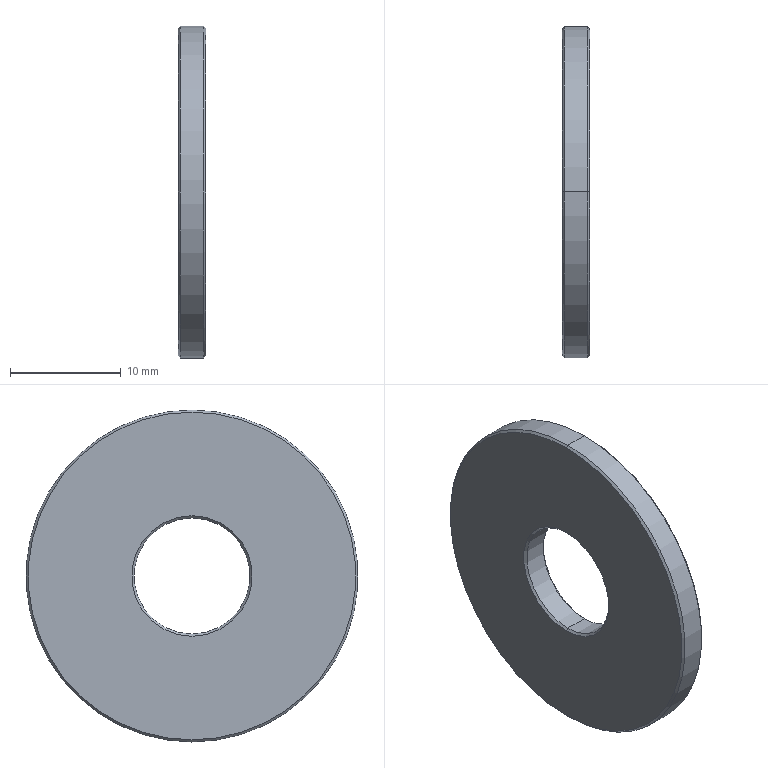Part | STEP file | WSX-SUS-M10X30-2.5-5 | 1 solid | 14 faces | box 2.5 x 30 x 30 mm | volume 1546 mm3 | cone 8 | cylinder 4 | plane 2 | commonest cylinder face diameters 10.5 x2 30 x2
STEP:
#1=CARTESIAN_POINT('',(0.,0.,0.));
#2=DIRECTION('',(0.,0.,1.));
#3=DIRECTION('',(1.,0.,0.));
#4=AXIS2_PLACEMENT_3D('',#1,#2,#3);
#5=CARTESIAN_POINT('',(2.5,0.,-14.8));
#6=VERTEX_POINT('',#5);
#7=CARTESIAN_POINT('',(2.5,0.,14.8));
#8=VERTEX_POINT('',#7);
#9=CARTESIAN_POINT('',(2.5,0.,0.));
#10=DIRECTION('',(1.,0.,0.));
#11=DIRECTION('',(0.,0.,1.));
#12=AXIS2_PLACEMENT_3D('',#9,#10,#11);
#13=CIRCLE('',#12,14.8);
#14=CARTESIAN_POINT('',(2.3,0.,0.));
#15=DIRECTION('',(-1.,0.,0.));
#16=DIRECTION('',(0.,0.,1.));
#17=AXIS2_PLACEMENT_3D('',#14,#15,#16);
#18=CONICAL_SURFACE('',#17,15.,0.7854);
#19=CARTESIAN_POINT('',(6.283,-0.2));
#20=DIRECTION('',(-1.,0.));
#21=VECTOR('',#20,1.);
#22=LINE('',#19,#21);
#23=(GEOMETRIC_REPRESENTATION_CONTEXT(2)PARAMETRIC_REPRESENTATION_CONTEXT()REPRESENTATION_CONTEXT('',''));
#24=DEFINITIONAL_REPRESENTATION('',(#22),#23);
#25=PCURVE('',#18,#24);
#26=CARTESIAN_POINT('',(2.5,5.,0.));
#27=DIRECTION('',(-1.,0.,0.));
#28=DIRECTION('',(0.,0.,1.));
#29=AXIS2_PLACEMENT_3D('',#26,#27,#28);
#30=PLANE('',#29);
#31=CARTESIAN_POINT('',(14.8,-5.));
#32=CARTESIAN_POINT('',(14.8,-30.634));
#33=CARTESIAN_POINT('',(-7.4,-17.817));
#34=CARTESIAN_POINT('',(-29.6,-5.));
#35=CARTESIAN_POINT('',(-7.4,7.817));
#36=CARTESIAN_POINT('',(14.8,20.634));
#37=CARTESIAN_POINT('',(14.8,-5.));
#38=(BOUNDED_CURVE()B_SPLINE_CURVE(2,(#31,#32,#33,#34,#35,#36,#37),.UNSPECIFIED.,.T.,.F.)B_SPLINE_CURVE_WITH_KNOTS((1,2,2,2,2,1),(-2.094,0.,2.094,4.189,6.283,8.378),.UNSPECIFIED.)CURVE()GEOMETRIC_REPRESENTATION_ITEM()RATIONAL_B_SPLINE_CURVE((1.,0.5,1.,0.5,1.,0.5,1.))REPRESENTATION_ITEM(''));
#39=(GEOMETRIC_REPRESENTATION_CONTEXT(2)PARAMETRIC_REPRESENTATION_CONTEXT()REPRESENTATION_CONTEXT('',''));
#40=DEFINITIONAL_REPRESENTATION('',(#38),#39);
#41=PCURVE('',#30,#40);
#42=SURFACE_CURVE('',#13,(#25,#41),.PCURVE_S1.);
#43=EDGE_CURVE('',#6,#8,#42,.T.);
#44=ORIENTED_EDGE('',*,*,#43,.F.);
#45=CARTESIAN_POINT('',(2.3,0.,-15.));
#46=VERTEX_POINT('',#45);
#47=CARTESIAN_POINT('',(2.3,0.,-15.));
#48=DIRECTION('',(-0.7071,0.,-0.7071));
#49=VECTOR('',#48,1.);
#50=LINE('',#47,#49);
#51=CARTESIAN_POINT('',(3.142,0.));
#52=DIRECTION('',(0.,1.));
#53=VECTOR('',#52,1.);
#54=LINE('',#51,#53);
#55=(GEOMETRIC_REPRESENTATION_CONTEXT(2)PARAMETRIC_REPRESENTATION_CONTEXT()REPRESENTATION_CONTEXT('',''));
#56=DEFINITIONAL_REPRESENTATION('',(#54),#55);
#57=PCURVE('',#18,#56);
#58=CARTESIAN_POINT('',(2.3,0.,0.));
#59=DIRECTION('',(-1.,0.,0.));
#60=DIRECTION('',(0.,0.,1.));
#61=AXIS2_PLACEMENT_3D('',#58,#59,#60);
#62=CONICAL_SURFACE('',#61,15.,0.7854);
#63=CARTESIAN_POINT('',(3.142,0.));
#64=DIRECTION('',(0.,1.));
#65=VECTOR('',#64,1.);
#66=LINE('',#63,#65);
#67=(GEOMETRIC_REPRESENTATION_CONTEXT(2)PARAMETRIC_REPRESENTATION_CONTEXT()REPRESENTATION_CONTEXT('',''));
#68=DEFINITIONAL_REPRESENTATION('',(#66),#67);
#69=PCURVE('',#62,#68);
#70=SURFACE_CURVE('',#50,(#57,#69),.PCURVE_S1.);
#71=EDGE_CURVE('',#6,#46,#70,.T.);
#72=ORIENTED_EDGE('',*,*,#71,.T.);
#73=CARTESIAN_POINT('',(2.3,0.,15.));
#74=VERTEX_POINT('',#73);
#75=CARTESIAN_POINT('',(2.3,0.,0.));
#76=DIRECTION('',(-1.,0.,0.));
#77=DIRECTION('',(0.,0.,1.));
#78=AXIS2_PLACEMENT_3D('',#75,#76,#77);
#79=CIRCLE('',#78,15.);
#80=CARTESIAN_POINT('',(0.,0.));
#81=DIRECTION('',(1.,0.));
#82=VECTOR('',#81,1.);
#83=LINE('',#80,#82);
#84=(GEOMETRIC_REPRESENTATION_CONTEXT(2)PARAMETRIC_REPRESENTATION_CONTEXT()REPRESENTATION_CONTEXT('',''));
#85=DEFINITIONAL_REPRESENTATION('',(#83),#84);
#86=PCURVE('',#18,#85);
#87=CARTESIAN_POINT('',(0.,0.,0.));
#88=DIRECTION('',(-1.,0.,0.));
#89=DIRECTION('',(0.,0.,1.));
#90=AXIS2_PLACEMENT_3D('',#87,#88,#89);
#91=CYLINDRICAL_SURFACE('',#90,15.);
#92=CARTESIAN_POINT('',(0.,-2.3));
#93=DIRECTION('',(1.,0.));
#94=VECTOR('',#93,1.);
#95=LINE('',#92,#94);
#96=(GEOMETRIC_REPRESENTATION_CONTEXT(2)PARAMETRIC_REPRESENTATION_CONTEXT()REPRESENTATION_CONTEXT('',''));
#97=DEFINITIONAL_REPRESENTATION('',(#95),#96);
#98=PCURVE('',#91,#97);
#99=SURFACE_CURVE('',#79,(#86,#98),.PCURVE_S1.);
#100=EDGE_CURVE('',#74,#46,#99,.T.);
#101=ORIENTED_EDGE('',*,*,#100,.F.);
#102=CARTESIAN_POINT('',(2.3,0.,15.));
#103=DIRECTION('',(-0.7071,0.,0.7071));
#104=VECTOR('',#103,1.);
#105=LINE('',#102,#104);
#106=CARTESIAN_POINT('',(0.,0.));
#107=DIRECTION('',(0.,1.));
#108=VECTOR('',#107,1.);
#109=LINE('',#106,#108);
#110=(GEOMETRIC_REPRESENTATION_CONTEXT(2)PARAMETRIC_REPRESENTATION_CONTEXT()REPRESENTATION_CONTEXT('',''));
#111=DEFINITIONAL_REPRESENTATION('',(#109),#110);
#112=PCURVE('',#18,#111);
#113=CARTESIAN_POINT('',(6.283,0.));
#114=DIRECTION('',(0.,1.));
#115=VECTOR('',#114,1.);
#116=LINE('',#113,#115);
#117=(GEOMETRIC_REPRESENTATION_CONTEXT(2)PARAMETRIC_REPRESENTATION_CONTEXT()REPRESENTATION_CONTEXT('',''));
#118=DEFINITIONAL_REPRESENTATION('',(#116),#117);
#119=PCURVE('',#62,#118);
#120=SURFACE_CURVE('',#105,(#112,#119),.PCURVE_S1.);
#121=EDGE_CURVE('',#8,#74,#120,.T.);
#122=ORIENTED_EDGE('',*,*,#121,.F.);
#123=EDGE_LOOP('',(#44,#72,#101,#122));
#124=FACE_BOUND('',#123,.T.);
#125=ADVANCED_FACE('',(#124),#18,.T.);
#126=CARTESIAN_POINT('',(2.3,0.,-5.25));
#127=VERTEX_POINT('',#126);
#128=CARTESIAN_POINT('',(2.5,0.,-5.45));
#129=VERTEX_POINT('',#128);
#130=CARTESIAN_POINT('',(2.5,0.,-5.45));
#131=DIRECTION('',(0.7071,0.,-0.7071));
#132=VECTOR('',#131,1.);
#133=LINE('',#130,#132);
#134=CARTESIAN_POINT('',(2.5,0.,0.));
#135=DIRECTION('',(1.,0.,0.));
#136=DIRECTION('',(0.,0.,-1.));
#137=AXIS2_PLACEMENT_3D('',#134,#135,#136);
#138=CONICAL_SURFACE('',#137,5.45,0.7854);
#139=CARTESIAN_POINT('',(6.283,0.));
#140=DIRECTION('',(0.,1.));
#141=VECTOR('',#140,1.);
#142=LINE('',#139,#141);
#143=(GEOMETRIC_REPRESENTATION_CONTEXT(2)PARAMETRIC_REPRESENTATION_CONTEXT()REPRESENTATION_CONTEXT('',''));
#144=DEFINITIONAL_REPRESENTATION('',(#142),#143);
#145=PCURVE('',#138,#144);
#146=CARTESIAN_POINT('',(2.5,0.,0.));
#147=DIRECTION('',(1.,0.,0.));
#148=DIRECTION('',(0.,0.,-1.));
#149=AXIS2_PLACEMENT_3D('',#146,#147,#148);
#150=CONICAL_SURFACE('',#149,5.45,0.7854);
#151=CARTESIAN_POINT('',(0.,0.));
#152=DIRECTION('',(0.,1.));
#153=VECTOR('',#152,1.);
#154=LINE('',#151,#153);
#155=(GEOMETRIC_REPRESENTATION_CONTEXT(2)PARAMETRIC_REPRESENTATION_CONTEXT()REPRESENTATION_CONTEXT('',''));
#156=DEFINITIONAL_REPRESENTATION('',(#154),#155);
#157=PCURVE('',#150,#156);
#158=SURFACE_CURVE('',#133,(#145,#157),.PCURVE_S1.);
#159=EDGE_CURVE('',#127,#129,#158,.T.);
#160=ORIENTED_EDGE('',*,*,#159,.T.);
#161=CARTESIAN_POINT('',(2.5,0.,5.45));
#162=VERTEX_POINT('',#161);
#163=CARTESIAN_POINT('',(2.5,0.,0.));
#164=DIRECTION('',(-1.,0.,0.));
#165=DIRECTION('',(0.,0.,1.));
#166=AXIS2_PLACEMENT_3D('',#163,#164,#165);
#167=CIRCLE('',#166,5.45);
#168=CARTESIAN_POINT('',(9.425,0.));
#169=DIRECTION('',(-1.,0.));
#170=VECTOR('',#169,1.);
#171=LINE('',#168,#170);
#172=(GEOMETRIC_REPRESENTATION_CONTEXT(2)PARAMETRIC_REPRESENTATION_CONTEXT()REPRESENTATION_CONTEXT('',''));
#173=DEFINITIONAL_REPRESENTATION('',(#171),#172);
#174=PCURVE('',#138,#173);
#175=CARTESIAN_POINT('',(0.,-5.));
#176=DIRECTION('',(1.,0.));
#177=AXIS2_PLACEMENT_2D('',#175,#176);
#178=CIRCLE('',#177,5.45);
#179=(GEOMETRIC_REPRESENTATION_CONTEXT(2)PARAMETRIC_REPRESENTATION_CONTEXT()REPRESENTATION_CONTEXT('',''));
#180=DEFINITIONAL_REPRESENTATION('',(#178),#179);
#181=PCURVE('',#30,#180);
#182=SURFACE_CURVE('',#167,(#174,#181),.PCURVE_S1.);
#183=EDGE_CURVE('',#129,#162,#182,.T.);
#184=ORIENTED_EDGE('',*,*,#183,.T.);
#185=CARTESIAN_POINT('',(2.3,0.,5.25));
#186=VERTEX_POINT('',#185);
#187=CARTESIAN_POINT('',(2.5,0.,5.45));
#188=DIRECTION('',(0.7071,0.,0.7071));
#189=VECTOR('',#188,1.);
#190=LINE('',#187,#189);
#191=CARTESIAN_POINT('',(3.142,0.));
#192=DIRECTION('',(0.,1.));
#193=VECTOR('',#192,1.);
#194=LINE('',#191,#193);
#195=(GEOMETRIC_REPRESENTATION_CONTEXT(2)PARAMETRIC_REPRESENTATION_CONTEXT()REPRESENTATION_CONTEXT('',''));
#196=DEFINITIONAL_REPRESENTATION('',(#194),#195);
#197=PCURVE('',#138,#196);
#198=CARTESIAN_POINT('',(3.142,0.));
#199=DIRECTION('',(0.,1.));
#200=VECTOR('',#199,1.);
#201=LINE('',#198,#200);
#202=(GEOMETRIC_REPRESENTATION_CONTEXT(2)PARAMETRIC_REPRESENTATION_CONTEXT()REPRESENTATION_CONTEXT('',''));
#203=DEFINITIONAL_REPRESENTATION('',(#201),#202);
#204=PCURVE('',#150,#203);
#205=SURFACE_CURVE('',#190,(#197,#204),.PCURVE_S1.);
#206=EDGE_CURVE('',#186,#162,#205,.T.);
#207=ORIENTED_EDGE('',*,*,#206,.F.);
#208=CARTESIAN_POINT('',(2.3,0.,0.));
#209=DIRECTION('',(1.,0.,0.));
#210=DIRECTION('',(0.,0.,-1.));
#211=AXIS2_PLACEMENT_3D('',#208,#209,#210);
#212=CIRCLE('',#211,5.25);
#213=CARTESIAN_POINT('',(0.,-0.2));
#214=DIRECTION('',(1.,0.));
#215=VECTOR('',#214,1.);
#216=LINE('',#213,#215);
#217=(GEOMETRIC_REPRESENTATION_CONTEXT(2)PARAMETRIC_REPRESENTATION_CONTEXT()REPRESENTATION_CONTEXT('',''));
#218=DEFINITIONAL_REPRESENTATION('',(#216),#217);
#219=PCURVE('',#138,#218);
#220=CARTESIAN_POINT('',(0.,0.,0.));
#221=DIRECTION('',(-1.,0.,0.));
#222=DIRECTION('',(0.,0.,1.));
#223=AXIS2_PLACEMENT_3D('',#220,#221,#222);
#224=CYLINDRICAL_SURFACE('',#223,5.25);
#225=CARTESIAN_POINT('',(9.425,-2.3));
#226=DIRECTION('',(-1.,0.));
#227=VECTOR('',#226,1.);
#228=LINE('',#225,#227);
#229=(GEOMETRIC_REPRESENTATION_CONTEXT(2)PARAMETRIC_REPRESENTATION_CONTEXT()REPRESENTATION_CONTEXT('',''));
#230=DEFINITIONAL_REPRESENTATION('',(#228),#229);
#231=PCURVE('',#224,#230);
#232=SURFACE_CURVE('',#212,(#219,#231),.PCURVE_S1.);
#233=EDGE_CURVE('',#186,#127,#232,.T.);
#234=ORIENTED_EDGE('',*,*,#233,.T.);
#235=EDGE_LOOP('',(#160,#184,#207,#234));
#236=FACE_BOUND('',#235,.F.);
#237=ADVANCED_FACE('',(#236),#138,.F.);
#238=CARTESIAN_POINT('',(0.,0.,14.8));
#239=VERTEX_POINT('',#238);
#240=CARTESIAN_POINT('',(0.,0.,-14.8));
#241=VERTEX_POINT('',#240);
#242=CARTESIAN_POINT('',(0.,0.,0.));
#243=DIRECTION('',(-1.,0.,0.));
#244=DIRECTION('',(0.,0.,-1.));
#245=AXIS2_PLACEMENT_3D('',#242,#243,#244);
#246=CIRCLE('',#245,14.8);
#247=CARTESIAN_POINT('',(0.,0.,0.));
#248=DIRECTION('',(1.,0.,0.));
#249=DIRECTION('',(0.,0.,-1.));
#250=AXIS2_PLACEMENT_3D('',#247,#248,#249);
#251=CONICAL_SURFACE('',#250,14.8,0.7854);
#252=CARTESIAN_POINT('',(6.283,0.));
#253=DIRECTION('',(-1.,0.));
#254=VECTOR('',#253,1.);
#255=LINE('',#252,#254);
#256=(GEOMETRIC_REPRESENTATION_CONTEXT(2)PARAMETRIC_REPRESENTATION_CONTEXT()REPRESENTATION_CONTEXT('',''));
#257=DEFINITIONAL_REPRESENTATION('',(#255),#256);
#258=PCURVE('',#251,#257);
#259=CARTESIAN_POINT('',(0.,5.,0.));
#260=DIRECTION('',(1.,0.,0.));
#261=DIRECTION('',(0.,0.,-1.));
#262=AXIS2_PLACEMENT_3D('',#259,#260,#261);
#263=PLANE('',#262);
#264=CARTESIAN_POINT('',(14.8,-5.));
#265=CARTESIAN_POINT('',(14.8,-30.634));
#266=CARTESIAN_POINT('',(-7.4,-17.817));
#267=CARTESIAN_POINT('',(-29.6,-5.));
#268=CARTESIAN_POINT('',(-7.4,7.817));
#269=CARTESIAN_POINT('',(14.8,20.634));
#270=CARTESIAN_POINT('',(14.8,-5.));
#271=(BOUNDED_CURVE()B_SPLINE_CURVE(2,(#264,#265,#266,#267,#268,#269,#270),.UNSPECIFIED.,.T.,.F.)B_SPLINE_CURVE_WITH_KNOTS((1,2,2,2,2,1),(-2.094,0.,2.094,4.189,6.283,8.378),.UNSPECIFIED.)CURVE()GEOMETRIC_REPRESENTATION_ITEM()RATIONAL_B_SPLINE_CURVE((1.,0.5,1.,0.5,1.,0.5,1.))REPRESENTATION_ITEM(''));
#272=(GEOMETRIC_REPRESENTATION_CONTEXT(2)PARAMETRIC_REPRESENTATION_CONTEXT()REPRESENTATION_CONTEXT('',''));
#273=DEFINITIONAL_REPRESENTATION('',(#271),#272);
#274=PCURVE('',#263,#273);
#275=SURFACE_CURVE('',#246,(#258,#274),.PCURVE_S1.);
#276=EDGE_CURVE('',#239,#241,#275,.T.);
#277=ORIENTED_EDGE('',*,*,#276,.F.);
#278=CARTESIAN_POINT('',(0.2,0.,15.));
#279=VERTEX_POINT('',#278);
#280=CARTESIAN_POINT('',(0.,0.,14.8));
#281=DIRECTION('',(0.7071,0.,0.7071));
#282=VECTOR('',#281,1.);
#283=LINE('',#280,#282);
#284=CARTESIAN_POINT('',(3.142,0.));
#285=DIRECTION('',(0.,1.));
#286=VECTOR('',#285,1.);
#287=LINE('',#284,#286);
#288=(GEOMETRIC_REPRESENTATION_CONTEXT(2)PARAMETRIC_REPRESENTATION_CONTEXT()REPRESENTATION_CONTEXT('',''));
#289=DEFINITIONAL_REPRESENTATION('',(#287),#288);
#290=PCURVE('',#251,#289);
#291=CARTESIAN_POINT('',(0.,0.,0.));
#292=DIRECTION('',(1.,0.,0.));
#293=DIRECTION('',(0.,0.,-1.));
#294=AXIS2_PLACEMENT_3D('',#291,#292,#293);
#295=CONICAL_SURFACE('',#294,14.8,0.7854);
#296=CARTESIAN_POINT('',(3.142,0.));
#297=DIRECTION('',(0.,1.));
#298=VECTOR('',#297,1.);
#299=LINE('',#296,#298);
#300=(GEOMETRIC_REPRESENTATION_CONTEXT(2)PARAMETRIC_REPRESENTATION_CONTEXT()REPRESENTATION_CONTEXT('',''));
#301=DEFINITIONAL_REPRESENTATION('',(#299),#300);
#302=PCURVE('',#295,#301);
#303=SURFACE_CURVE('',#283,(#290,#302),.PCURVE_S1.);
#304=EDGE_CURVE('',#239,#279,#303,.T.);
#305=ORIENTED_EDGE('',*,*,#304,.T.);
#306=CARTESIAN_POINT('',(0.2,0.,-15.));
#307=VERTEX_POINT('',#306);
#308=CARTESIAN_POINT('',(0.2,0.,0.));
#309=DIRECTION('',(1.,0.,0.));
#310=DIRECTION('',(0.,0.,-1.));
#311=AXIS2_PLACEMENT_3D('',#308,#309,#310);
#312=CIRCLE('',#311,15.);
#313=CARTESIAN_POINT('',(0.,0.2));
#314=DIRECTION('',(1.,0.));
#315=VECTOR('',#314,1.);
#316=LINE('',#313,#315);
#317=(GEOMETRIC_REPRESENTATION_CONTEXT(2)PARAMETRIC_REPRESENTATION_CONTEXT()REPRESENTATION_CONTEXT('',''));
#318=DEFINITIONAL_REPRESENTATION('',(#316),#317);
#319=PCURVE('',#251,#318);
#320=CARTESIAN_POINT('',(3.142,-0.2));
#321=DIRECTION('',(-1.,0.));
#322=VECTOR('',#321,1.);
#323=LINE('',#320,#322);
#324=(GEOMETRIC_REPRESENTATION_CONTEXT(2)PARAMETRIC_REPRESENTATION_CONTEXT()REPRESENTATION_CONTEXT('',''));
#325=DEFINITIONAL_REPRESENTATION('',(#323),#324);
#326=PCURVE('',#91,#325);
#327=SURFACE_CURVE('',#312,(#319,#326),.PCURVE_S1.);
#328=EDGE_CURVE('',#307,#279,#327,.T.);
#329=ORIENTED_EDGE('',*,*,#328,.F.);
#330=CARTESIAN_POINT('',(0.,0.,-14.8));
#331=DIRECTION('',(0.7071,0.,-0.7071));
#332=VECTOR('',#331,1.);
#333=LINE('',#330,#332);
#334=CARTESIAN_POINT('',(0.,0.));
#335=DIRECTION('',(0.,1.));
#336=VECTOR('',#335,1.);
#337=LINE('',#334,#336);
#338=(GEOMETRIC_REPRESENTATION_CONTEXT(2)PARAMETRIC_REPRESENTATION_CONTEXT()REPRESENTATION_CONTEXT('',''));
#339=DEFINITIONAL_REPRESENTATION('',(#337),#338);
#340=PCURVE('',#251,#339);
#341=CARTESIAN_POINT('',(6.283,0.));
#342=DIRECTION('',(0.,1.));
#343=VECTOR('',#342,1.);
#344=LINE('',#341,#343);
#345=(GEOMETRIC_REPRESENTATION_CONTEXT(2)PARAMETRIC_REPRESENTATION_CONTEXT()REPRESENTATION_CONTEXT('',''));
#346=DEFINITIONAL_REPRESENTATION('',(#344),#345);
#347=PCURVE('',#295,#346);
#348=SURFACE_CURVE('',#333,(#340,#347),.PCURVE_S1.);
#349=EDGE_CURVE('',#241,#307,#348,.T.);
#350=ORIENTED_EDGE('',*,*,#349,.F.);
#351=EDGE_LOOP('',(#277,#305,#329,#350));
#352=FACE_BOUND('',#351,.T.);
#353=ADVANCED_FACE('',(#352),#251,.T.);
#354=CARTESIAN_POINT('',(0.2,0.,5.25));
#355=VERTEX_POINT('',#354);
#356=CARTESIAN_POINT('',(0.,0.,5.45));
#357=VERTEX_POINT('',#356);
#358=CARTESIAN_POINT('',(0.2,0.,5.25));
#359=DIRECTION('',(-0.7071,0.,0.7071));
#360=VECTOR('',#359,1.);
#361=LINE('',#358,#360);
#362=CARTESIAN_POINT('',(0.2,0.,0.));
#363=DIRECTION('',(-1.,0.,0.));
#364=DIRECTION('',(0.,0.,1.));
#365=AXIS2_PLACEMENT_3D('',#362,#363,#364);
#366=CONICAL_SURFACE('',#365,5.25,0.7854);
#367=CARTESIAN_POINT('',(6.283,0.));
#368=DIRECTION('',(0.,1.));
#369=VECTOR('',#368,1.);
#370=LINE('',#367,#369);
#371=(GEOMETRIC_REPRESENTATION_CONTEXT(2)PARAMETRIC_REPRESENTATION_CONTEXT()REPRESENTATION_CONTEXT('',''));
#372=DEFINITIONAL_REPRESENTATION('',(#370),#371);
#373=PCURVE('',#366,#372);
#374=CARTESIAN_POINT('',(0.2,0.,0.));
#375=DIRECTION('',(-1.,0.,0.));
#376=DIRECTION('',(0.,0.,1.));
#377=AXIS2_PLACEMENT_3D('',#374,#375,#376);
#378=CONICAL_SURFACE('',#377,5.25,0.7854);
#379=CARTESIAN_POINT('',(0.,0.));
#380=DIRECTION('',(0.,1.));
#381=VECTOR('',#380,1.);
#382=LINE('',#379,#381);
#383=(GEOMETRIC_REPRESENTATION_CONTEXT(2)PARAMETRIC_REPRESENTATION_CONTEXT()REPRESENTATION_CONTEXT('',''));
#384=DEFINITIONAL_REPRESENTATION('',(#382),#383);
#385=PCURVE('',#378,#384);
#386=SURFACE_CURVE('',#361,(#373,#385),.PCURVE_S1.);
#387=EDGE_CURVE('',#355,#357,#386,.T.);
#388=ORIENTED_EDGE('',*,*,#387,.T.);
#389=CARTESIAN_POINT('',(0.,0.,-5.45));
#390=VERTEX_POINT('',#389);
#391=CARTESIAN_POINT('',(0.,0.,0.));
#392=DIRECTION('',(1.,0.,0.));
#393=DIRECTION('',(0.,0.,-1.));
#394=AXIS2_PLACEMENT_3D('',#391,#392,#393);
#395=CIRCLE('',#394,5.45);
#396=CARTESIAN_POINT('',(9.425,0.2));
#397=DIRECTION('',(-1.,0.));
#398=VECTOR('',#397,1.);
#399=LINE('',#396,#398);
#400=(GEOMETRIC_REPRESENTATION_CONTEXT(2)PARAMETRIC_REPRESENTATION_CONTEXT()REPRESENTATION_CONTEXT('',''));
#401=DEFINITIONAL_REPRESENTATION('',(#399),#400);
#402=PCURVE('',#366,#401);
#403=CARTESIAN_POINT('',(0.,-5.));
#404=DIRECTION('',(1.,0.));
#405=AXIS2_PLACEMENT_2D('',#403,#404);
#406=CIRCLE('',#405,5.45);
#407=(GEOMETRIC_REPRESENTATION_CONTEXT(2)PARAMETRIC_REPRESENTATION_CONTEXT()REPRESENTATION_CONTEXT('',''));
#408=DEFINITIONAL_REPRESENTATION('',(#406),#407);
#409=PCURVE('',#263,#408);
#410=SURFACE_CURVE('',#395,(#402,#409),.PCURVE_S1.);
#411=EDGE_CURVE('',#357,#390,#410,.T.);
#412=ORIENTED_EDGE('',*,*,#411,.T.);
#413=CARTESIAN_POINT('',(0.2,0.,-5.25));
#414=VERTEX_POINT('',#413);
#415=CARTESIAN_POINT('',(0.2,0.,-5.25));
#416=DIRECTION('',(-0.7071,0.,-0.7071));
#417=VECTOR('',#416,1.);
#418=LINE('',#415,#417);
#419=CARTESIAN_POINT('',(3.142,0.));
#420=DIRECTION('',(0.,1.));
#421=VECTOR('',#420,1.);
#422=LINE('',#419,#421);
#423=(GEOMETRIC_REPRESENTATION_CONTEXT(2)PARAMETRIC_REPRESENTATION_CONTEXT()REPRESENTATION_CONTEXT('',''));
#424=DEFINITIONAL_REPRESENTATION('',(#422),#423);
#425=PCURVE('',#366,#424);
#426=CARTESIAN_POINT('',(3.142,0.));
#427=DIRECTION('',(0.,1.));
#428=VECTOR('',#427,1.);
#429=LINE('',#426,#428);
#430=(GEOMETRIC_REPRESENTATION_CONTEXT(2)PARAMETRIC_REPRESENTATION_CONTEXT()REPRESENTATION_CONTEXT('',''));
#431=DEFINITIONAL_REPRESENTATION('',(#429),#430);
#432=PCURVE('',#378,#431);
#433=SURFACE_CURVE('',#418,(#425,#432),.PCURVE_S1.);
#434=EDGE_CURVE('',#414,#390,#433,.T.);
#435=ORIENTED_EDGE('',*,*,#434,.F.);
#436=CARTESIAN_POINT('',(0.2,0.,0.));
#437=DIRECTION('',(-1.,0.,0.));
#438=DIRECTION('',(0.,0.,1.));
#439=AXIS2_PLACEMENT_3D('',#436,#437,#438);
#440=CIRCLE('',#439,5.25);
#441=CARTESIAN_POINT('',(0.,0.));
#442=DIRECTION('',(1.,0.));
#443=VECTOR('',#442,1.);
#444=LINE('',#441,#443);
#445=(GEOMETRIC_REPRESENTATION_CONTEXT(2)PARAMETRIC_REPRESENTATION_CONTEXT()REPRESENTATION_CONTEXT('',''));
#446=DEFINITIONAL_REPRESENTATION('',(#444),#445);
#447=PCURVE('',#366,#446);
#448=CARTESIAN_POINT('',(0.,-0.2));
#449=DIRECTION('',(1.,0.));
#450=VECTOR('',#449,1.);
#451=LINE('',#448,#450);
#452=(GEOMETRIC_REPRESENTATION_CONTEXT(2)PARAMETRIC_REPRESENTATION_CONTEXT()REPRESENTATION_CONTEXT('',''));
#453=DEFINITIONAL_REPRESENTATION('',(#451),#452);
#454=PCURVE('',#224,#453);
#455=SURFACE_CURVE('',#440,(#447,#454),.PCURVE_S1.);
#456=EDGE_CURVE('',#414,#355,#455,.T.);
#457=ORIENTED_EDGE('',*,*,#456,.T.);
#458=EDGE_LOOP('',(#388,#412,#435,#457));
#459=FACE_BOUND('',#458,.F.);
#460=ADVANCED_FACE('',(#459),#366,.F.);
#461=CARTESIAN_POINT('',(0.,0.,5.25));
#462=DIRECTION('',(-1.,0.,0.));
#463=VECTOR('',#462,1.);
#464=LINE('',#461,#463);
#465=CARTESIAN_POINT('',(6.283,0.));
#466=DIRECTION('',(0.,1.));
#467=VECTOR('',#466,1.);
#468=LINE('',#465,#467);
#469=(GEOMETRIC_REPRESENTATION_CONTEXT(2)PARAMETRIC_REPRESENTATION_CONTEXT()REPRESENTATION_CONTEXT('',''));
#470=DEFINITIONAL_REPRESENTATION('',(#468),#469);
#471=PCURVE('',#224,#470);
#472=CARTESIAN_POINT('',(0.,0.,0.));
#473=DIRECTION('',(-1.,0.,0.));
#474=DIRECTION('',(0.,0.,1.));
#475=AXIS2_PLACEMENT_3D('',#472,#473,#474);
#476=CYLINDRICAL_SURFACE('',#475,5.25);
#477=CARTESIAN_POINT('',(0.,0.));
#478=DIRECTION('',(0.,1.));
#479=VECTOR('',#478,1.);
#480=LINE('',#477,#479);
#481=(GEOMETRIC_REPRESENTATION_CONTEXT(2)PARAMETRIC_REPRESENTATION_CONTEXT()REPRESENTATION_CONTEXT('',''));
#482=DEFINITIONAL_REPRESENTATION('',(#480),#481);
#483=PCURVE('',#476,#482);
#484=SURFACE_CURVE('',#464,(#471,#483),.PCURVE_S1.);
#485=EDGE_CURVE('',#186,#355,#484,.T.);
#486=ORIENTED_EDGE('',*,*,#485,.T.);
#487=ORIENTED_EDGE('',*,*,#456,.F.);
#488=CARTESIAN_POINT('',(0.,0.,-5.25));
#489=DIRECTION('',(-1.,0.,0.));
#490=VECTOR('',#489,1.);
#491=LINE('',#488,#490);
#492=CARTESIAN_POINT('',(3.142,0.));
#493=DIRECTION('',(0.,1.));
#494=VECTOR('',#493,1.);
#495=LINE('',#492,#494);
#496=(GEOMETRIC_REPRESENTATION_CONTEXT(2)PARAMETRIC_REPRESENTATION_CONTEXT()REPRESENTATION_CONTEXT('',''));
#497=DEFINITIONAL_REPRESENTATION('',(#495),#496);
#498=PCURVE('',#224,#497);
#499=CARTESIAN_POINT('',(3.142,0.));
#500=DIRECTION('',(0.,1.));
#501=VECTOR('',#500,1.);
#502=LINE('',#499,#501);
#503=(GEOMETRIC_REPRESENTATION_CONTEXT(2)PARAMETRIC_REPRESENTATION_CONTEXT()REPRESENTATION_CONTEXT('',''));
#504=DEFINITIONAL_REPRESENTATION('',(#502),#503);
#505=PCURVE('',#476,#504);
#506=SURFACE_CURVE('',#491,(#498,#505),.PCURVE_S1.);
#507=EDGE_CURVE('',#127,#414,#506,.T.);
#508=ORIENTED_EDGE('',*,*,#507,.F.);
#509=ORIENTED_EDGE('',*,*,#233,.F.);
#510=EDGE_LOOP('',(#486,#487,#508,#509));
#511=FACE_BOUND('',#510,.F.);
#512=ADVANCED_FACE('',(#511),#224,.F.);
#513=ORIENTED_EDGE('',*,*,#100,.T.);
#514=CARTESIAN_POINT('',(0.,0.,-15.));
#515=DIRECTION('',(-1.,0.,0.));
#516=VECTOR('',#515,1.);
#517=LINE('',#514,#516);
#518=CARTESIAN_POINT('',(3.142,0.));
#519=DIRECTION('',(0.,1.));
#520=VECTOR('',#519,1.);
#521=LINE('',#518,#520);
#522=(GEOMETRIC_REPRESENTATION_CONTEXT(2)PARAMETRIC_REPRESENTATION_CONTEXT()REPRESENTATION_CONTEXT('',''));
#523=DEFINITIONAL_REPRESENTATION('',(#521),#522);
#524=PCURVE('',#91,#523);
#525=CARTESIAN_POINT('',(0.,0.,0.));
#526=DIRECTION('',(-1.,0.,0.));
#527=DIRECTION('',(0.,0.,1.));
#528=AXIS2_PLACEMENT_3D('',#525,#526,#527);
#529=CYLINDRICAL_SURFACE('',#528,15.);
#530=CARTESIAN_POINT('',(3.142,0.));
#531=DIRECTION('',(0.,1.));
#532=VECTOR('',#531,1.);
#533=LINE('',#530,#532);
#534=(GEOMETRIC_REPRESENTATION_CONTEXT(2)PARAMETRIC_REPRESENTATION_CONTEXT()REPRESENTATION_CONTEXT('',''));
#535=DEFINITIONAL_REPRESENTATION('',(#533),#534);
#536=PCURVE('',#529,#535);
#537=SURFACE_CURVE('',#517,(#524,#536),.PCURVE_S1.);
#538=EDGE_CURVE('',#46,#307,#537,.T.);
#539=ORIENTED_EDGE('',*,*,#538,.T.);
#540=ORIENTED_EDGE('',*,*,#328,.T.);
#541=CARTESIAN_POINT('',(0.,0.,15.));
#542=DIRECTION('',(-1.,0.,0.));
#543=VECTOR('',#542,1.);
#544=LINE('',#541,#543);
#545=CARTESIAN_POINT('',(0.,0.));
#546=DIRECTION('',(0.,1.));
#547=VECTOR('',#546,1.);
#548=LINE('',#545,#547);
#549=(GEOMETRIC_REPRESENTATION_CONTEXT(2)PARAMETRIC_REPRESENTATION_CONTEXT()REPRESENTATION_CONTEXT('',''));
#550=DEFINITIONAL_REPRESENTATION('',(#548),#549);
#551=PCURVE('',#91,#550);
#552=CARTESIAN_POINT('',(6.283,0.));
#553=DIRECTION('',(0.,1.));
#554=VECTOR('',#553,1.);
#555=LINE('',#552,#554);
#556=(GEOMETRIC_REPRESENTATION_CONTEXT(2)PARAMETRIC_REPRESENTATION_CONTEXT()REPRESENTATION_CONTEXT('',''));
#557=DEFINITIONAL_REPRESENTATION('',(#555),#556);
#558=PCURVE('',#529,#557);
#559=SURFACE_CURVE('',#544,(#551,#558),.PCURVE_S1.);
#560=EDGE_CURVE('',#74,#279,#559,.T.);
#561=ORIENTED_EDGE('',*,*,#560,.F.);
#562=EDGE_LOOP('',(#513,#539,#540,#561));
#563=FACE_BOUND('',#562,.T.);
#564=ADVANCED_FACE('',(#563),#91,.T.);
#565=ORIENTED_EDGE('',*,*,#411,.T.);
#566=CARTESIAN_POINT('',(0.,0.,0.));
#567=DIRECTION('',(1.,0.,0.));
#568=DIRECTION('',(0.,0.,-1.));
#569=AXIS2_PLACEMENT_3D('',#566,#567,#568);
#570=CIRCLE('',#569,5.45);
#571=CARTESIAN_POINT('',(0.,-5.));
#572=DIRECTION('',(1.,0.));
#573=AXIS2_PLACEMENT_2D('',#571,#572);
#574=CIRCLE('',#573,5.45);
#575=(GEOMETRIC_REPRESENTATION_CONTEXT(2)PARAMETRIC_REPRESENTATION_CONTEXT()REPRESENTATION_CONTEXT('',''));
#576=DEFINITIONAL_REPRESENTATION('',(#574),#575);
#577=PCURVE('',#263,#576);
#578=CARTESIAN_POINT('',(3.142,0.2));
#579=DIRECTION('',(-1.,0.));
#580=VECTOR('',#579,1.);
#581=LINE('',#578,#580);
#582=(GEOMETRIC_REPRESENTATION_CONTEXT(2)PARAMETRIC_REPRESENTATION_CONTEXT()REPRESENTATION_CONTEXT('',''));
#583=DEFINITIONAL_REPRESENTATION('',(#581),#582);
#584=PCURVE('',#378,#583);
#585=SURFACE_CURVE('',#570,(#577,#584),.PCURVE_S1.);
#586=EDGE_CURVE('',#390,#357,#585,.T.);
#587=ORIENTED_EDGE('',*,*,#586,.T.);
#588=EDGE_LOOP('',(#565,#587));
#589=FACE_BOUND('',#588,.T.);
#590=CARTESIAN_POINT('',(0.,0.,0.));
#591=DIRECTION('',(-1.,0.,0.));
#592=DIRECTION('',(0.,0.,-1.));
#593=AXIS2_PLACEMENT_3D('',#590,#591,#592);
#594=CIRCLE('',#593,14.8);
#595=CARTESIAN_POINT('',(14.8,-5.));
#596=CARTESIAN_POINT('',(14.8,-30.634));
#597=CARTESIAN_POINT('',(-7.4,-17.817));
#598=CARTESIAN_POINT('',(-29.6,-5.));
#599=CARTESIAN_POINT('',(-7.4,7.817));
#600=CARTESIAN_POINT('',(14.8,20.634));
#601=CARTESIAN_POINT('',(14.8,-5.));
#602=(BOUNDED_CURVE()B_SPLINE_CURVE(2,(#595,#596,#597,#598,#599,#600,#601),.UNSPECIFIED.,.T.,.F.)B_SPLINE_CURVE_WITH_KNOTS((1,2,2,2,2,1),(-2.094,0.,2.094,4.189,6.283,8.378),.UNSPECIFIED.)CURVE()GEOMETRIC_REPRESENTATION_ITEM()RATIONAL_B_SPLINE_CURVE((1.,0.5,1.,0.5,1.,0.5,1.))REPRESENTATION_ITEM(''));
#603=(GEOMETRIC_REPRESENTATION_CONTEXT(2)PARAMETRIC_REPRESENTATION_CONTEXT()REPRESENTATION_CONTEXT('',''));
#604=DEFINITIONAL_REPRESENTATION('',(#602),#603);
#605=PCURVE('',#263,#604);
#606=CARTESIAN_POINT('',(6.283,0.));
#607=DIRECTION('',(-1.,0.));
#608=VECTOR('',#607,1.);
#609=LINE('',#606,#608);
#610=(GEOMETRIC_REPRESENTATION_CONTEXT(2)PARAMETRIC_REPRESENTATION_CONTEXT()REPRESENTATION_CONTEXT('',''));
#611=DEFINITIONAL_REPRESENTATION('',(#609),#610);
#612=PCURVE('',#295,#611);
#613=SURFACE_CURVE('',#594,(#605,#612),.PCURVE_S1.);
#614=EDGE_CURVE('',#241,#239,#613,.T.);
#615=ORIENTED_EDGE('',*,*,#614,.T.);
#616=ORIENTED_EDGE('',*,*,#276,.T.);
#617=EDGE_LOOP('',(#615,#616));
#618=FACE_BOUND('',#617,.T.);
#619=ADVANCED_FACE('',(#589,#618),#263,.F.);
#620=ORIENTED_EDGE('',*,*,#538,.F.);
#621=CARTESIAN_POINT('',(2.3,0.,0.));
#622=DIRECTION('',(-1.,0.,0.));
#623=DIRECTION('',(0.,0.,1.));
#624=AXIS2_PLACEMENT_3D('',#621,#622,#623);
#625=CIRCLE('',#624,15.);
#626=CARTESIAN_POINT('',(0.,-2.3));
#627=DIRECTION('',(1.,0.));
#628=VECTOR('',#627,1.);
#629=LINE('',#626,#628);
#630=(GEOMETRIC_REPRESENTATION_CONTEXT(2)PARAMETRIC_REPRESENTATION_CONTEXT()REPRESENTATION_CONTEXT('',''));
#631=DEFINITIONAL_REPRESENTATION('',(#629),#630);
#632=PCURVE('',#529,#631);
#633=CARTESIAN_POINT('',(0.,0.));
#634=DIRECTION('',(1.,0.));
#635=VECTOR('',#634,1.);
#636=LINE('',#633,#635);
#637=(GEOMETRIC_REPRESENTATION_CONTEXT(2)PARAMETRIC_REPRESENTATION_CONTEXT()REPRESENTATION_CONTEXT('',''));
#638=DEFINITIONAL_REPRESENTATION('',(#636),#637);
#639=PCURVE('',#62,#638);
#640=SURFACE_CURVE('',#625,(#632,#639),.PCURVE_S1.);
#641=EDGE_CURVE('',#46,#74,#640,.T.);
#642=ORIENTED_EDGE('',*,*,#641,.T.);
#643=ORIENTED_EDGE('',*,*,#560,.T.);
#644=CARTESIAN_POINT('',(0.2,0.,0.));
#645=DIRECTION('',(1.,0.,0.));
#646=DIRECTION('',(0.,0.,-1.));
#647=AXIS2_PLACEMENT_3D('',#644,#645,#646);
#648=CIRCLE('',#647,15.);
#649=CARTESIAN_POINT('',(9.425,-0.2));
#650=DIRECTION('',(-1.,0.));
#651=VECTOR('',#650,1.);
#652=LINE('',#649,#651);
#653=(GEOMETRIC_REPRESENTATION_CONTEXT(2)PARAMETRIC_REPRESENTATION_CONTEXT()REPRESENTATION_CONTEXT('',''));
#654=DEFINITIONAL_REPRESENTATION('',(#652),#653);
#655=PCURVE('',#529,#654);
#656=CARTESIAN_POINT('',(0.,0.2));
#657=DIRECTION('',(1.,0.));
#658=VECTOR('',#657,1.);
#659=LINE('',#656,#658);
#660=(GEOMETRIC_REPRESENTATION_CONTEXT(2)PARAMETRIC_REPRESENTATION_CONTEXT()REPRESENTATION_CONTEXT('',''));
#661=DEFINITIONAL_REPRESENTATION('',(#659),#660);
#662=PCURVE('',#295,#661);
#663=SURFACE_CURVE('',#648,(#655,#662),.PCURVE_S1.);
#664=EDGE_CURVE('',#279,#307,#663,.T.);
#665=ORIENTED_EDGE('',*,*,#664,.T.);
#666=EDGE_LOOP('',(#620,#642,#643,#665));
#667=FACE_BOUND('',#666,.T.);
#668=ADVANCED_FACE('',(#667),#529,.T.);
#669=ORIENTED_EDGE('',*,*,#183,.T.);
#670=CARTESIAN_POINT('',(2.5,0.,0.));
#671=DIRECTION('',(-1.,0.,0.));
#672=DIRECTION('',(0.,0.,1.));
#673=AXIS2_PLACEMENT_3D('',#670,#671,#672);
#674=CIRCLE('',#673,5.45);
#675=CARTESIAN_POINT('',(0.,-5.));
#676=DIRECTION('',(1.,0.));
#677=AXIS2_PLACEMENT_2D('',#675,#676);
#678=CIRCLE('',#677,5.45);
#679=(GEOMETRIC_REPRESENTATION_CONTEXT(2)PARAMETRIC_REPRESENTATION_CONTEXT()REPRESENTATION_CONTEXT('',''));
#680=DEFINITIONAL_REPRESENTATION('',(#678),#679);
#681=PCURVE('',#30,#680);
#682=CARTESIAN_POINT('',(3.142,0.));
#683=DIRECTION('',(-1.,0.));
#684=VECTOR('',#683,1.);
#685=LINE('',#682,#684);
#686=(GEOMETRIC_REPRESENTATION_CONTEXT(2)PARAMETRIC_REPRESENTATION_CONTEXT()REPRESENTATION_CONTEXT('',''));
#687=DEFINITIONAL_REPRESENTATION('',(#685),#686);
#688=PCURVE('',#150,#687);
#689=SURFACE_CURVE('',#674,(#681,#688),.PCURVE_S1.);
#690=EDGE_CURVE('',#162,#129,#689,.T.);
#691=ORIENTED_EDGE('',*,*,#690,.T.);
#692=EDGE_LOOP('',(#669,#691));
#693=FACE_BOUND('',#692,.T.);
#694=CARTESIAN_POINT('',(2.5,0.,0.));
#695=DIRECTION('',(1.,0.,0.));
#696=DIRECTION('',(0.,0.,1.));
#697=AXIS2_PLACEMENT_3D('',#694,#695,#696);
#698=CIRCLE('',#697,14.8);
#699=CARTESIAN_POINT('',(14.8,-5.));
#700=CARTESIAN_POINT('',(14.8,-30.634));
#701=CARTESIAN_POINT('',(-7.4,-17.817));
#702=CARTESIAN_POINT('',(-29.6,-5.));
#703=CARTESIAN_POINT('',(-7.4,7.817));
#704=CARTESIAN_POINT('',(14.8,20.634));
#705=CARTESIAN_POINT('',(14.8,-5.));
#706=(BOUNDED_CURVE()B_SPLINE_CURVE(2,(#699,#700,#701,#702,#703,#704,#705),.UNSPECIFIED.,.T.,.F.)B_SPLINE_CURVE_WITH_KNOTS((1,2,2,2,2,1),(-2.094,0.,2.094,4.189,6.283,8.378),.UNSPECIFIED.)CURVE()GEOMETRIC_REPRESENTATION_ITEM()RATIONAL_B_SPLINE_CURVE((1.,0.5,1.,0.5,1.,0.5,1.))REPRESENTATION_ITEM(''));
#707=(GEOMETRIC_REPRESENTATION_CONTEXT(2)PARAMETRIC_REPRESENTATION_CONTEXT()REPRESENTATION_CONTEXT('',''));
#708=DEFINITIONAL_REPRESENTATION('',(#706),#707);
#709=PCURVE('',#30,#708);
#710=CARTESIAN_POINT('',(6.283,-0.2));
#711=DIRECTION('',(-1.,0.));
#712=VECTOR('',#711,1.);
#713=LINE('',#710,#712);
#714=(GEOMETRIC_REPRESENTATION_CONTEXT(2)PARAMETRIC_REPRESENTATION_CONTEXT()REPRESENTATION_CONTEXT('',''));
#715=DEFINITIONAL_REPRESENTATION('',(#713),#714);
#716=PCURVE('',#62,#715);
#717=SURFACE_CURVE('',#698,(#709,#716),.PCURVE_S1.);
#718=EDGE_CURVE('',#8,#6,#717,.T.);
#719=ORIENTED_EDGE('',*,*,#718,.T.);
#720=ORIENTED_EDGE('',*,*,#43,.T.);
#721=EDGE_LOOP('',(#719,#720));
#722=FACE_BOUND('',#721,.T.);
#723=ADVANCED_FACE('',(#693,#722),#30,.F.);
#724=CARTESIAN_POINT('',(0.2,0.,0.));
#725=DIRECTION('',(-1.,0.,0.));
#726=DIRECTION('',(0.,0.,1.));
#727=AXIS2_PLACEMENT_3D('',#724,#725,#726);
#728=CIRCLE('',#727,5.25);
#729=CARTESIAN_POINT('',(0.,-0.2));
#730=DIRECTION('',(1.,0.));
#731=VECTOR('',#730,1.);
#732=LINE('',#729,#731);
#733=(GEOMETRIC_REPRESENTATION_CONTEXT(2)PARAMETRIC_REPRESENTATION_CONTEXT()REPRESENTATION_CONTEXT('',''));
#734=DEFINITIONAL_REPRESENTATION('',(#732),#733);
#735=PCURVE('',#476,#734);
#736=CARTESIAN_POINT('',(0.,0.));
#737=DIRECTION('',(1.,0.));
#738=VECTOR('',#737,1.);
#739=LINE('',#736,#738);
#740=(GEOMETRIC_REPRESENTATION_CONTEXT(2)PARAMETRIC_REPRESENTATION_CONTEXT()REPRESENTATION_CONTEXT('',''));
#741=DEFINITIONAL_REPRESENTATION('',(#739),#740);
#742=PCURVE('',#378,#741);
#743=SURFACE_CURVE('',#728,(#735,#742),.PCURVE_S1.);
#744=EDGE_CURVE('',#355,#414,#743,.T.);
#745=ORIENTED_EDGE('',*,*,#744,.F.);
#746=ORIENTED_EDGE('',*,*,#485,.F.);
#747=CARTESIAN_POINT('',(2.3,0.,0.));
#748=DIRECTION('',(1.,0.,0.));
#749=DIRECTION('',(0.,0.,-1.));
#750=AXIS2_PLACEMENT_3D('',#747,#748,#749);
#751=CIRCLE('',#750,5.25);
#752=CARTESIAN_POINT('',(3.142,-2.3));
#753=DIRECTION('',(-1.,0.));
#754=VECTOR('',#753,1.);
#755=LINE('',#752,#754);
#756=(GEOMETRIC_REPRESENTATION_CONTEXT(2)PARAMETRIC_REPRESENTATION_CONTEXT()REPRESENTATION_CONTEXT('',''));
#757=DEFINITIONAL_REPRESENTATION('',(#755),#756);
#758=PCURVE('',#476,#757);
#759=CARTESIAN_POINT('',(0.,-0.2));
#760=DIRECTION('',(1.,0.));
#761=VECTOR('',#760,1.);
#762=LINE('',#759,#761);
#763=(GEOMETRIC_REPRESENTATION_CONTEXT(2)PARAMETRIC_REPRESENTATION_CONTEXT()REPRESENTATION_CONTEXT('',''));
#764=DEFINITIONAL_REPRESENTATION('',(#762),#763);
#765=PCURVE('',#150,#764);
#766=SURFACE_CURVE('',#751,(#758,#765),.PCURVE_S1.);
#767=EDGE_CURVE('',#127,#186,#766,.T.);
#768=ORIENTED_EDGE('',*,*,#767,.F.);
#769=ORIENTED_EDGE('',*,*,#507,.T.);
#770=EDGE_LOOP('',(#745,#746,#768,#769));
#771=FACE_BOUND('',#770,.F.);
#772=ADVANCED_FACE('',(#771),#476,.F.);
#773=ORIENTED_EDGE('',*,*,#586,.T.);
#774=ORIENTED_EDGE('',*,*,#387,.F.);
#775=ORIENTED_EDGE('',*,*,#744,.T.);
#776=ORIENTED_EDGE('',*,*,#434,.T.);
#777=EDGE_LOOP('',(#773,#774,#775,#776));
#778=FACE_BOUND('',#777,.F.);
#779=ADVANCED_FACE('',(#778),#378,.F.);
#780=ORIENTED_EDGE('',*,*,#304,.F.);
#781=ORIENTED_EDGE('',*,*,#614,.F.);
#782=ORIENTED_EDGE('',*,*,#349,.T.);
#783=ORIENTED_EDGE('',*,*,#664,.F.);
#784=EDGE_LOOP('',(#780,#781,#782,#783));
#785=FACE_BOUND('',#784,.T.);
#786=ADVANCED_FACE('',(#785),#295,.T.);
#787=ORIENTED_EDGE('',*,*,#690,.T.);
#788=ORIENTED_EDGE('',*,*,#159,.F.);
#789=ORIENTED_EDGE('',*,*,#767,.T.);
#790=ORIENTED_EDGE('',*,*,#206,.T.);
#791=EDGE_LOOP('',(#787,#788,#789,#790));
#792=FACE_BOUND('',#791,.F.);
#793=ADVANCED_FACE('',(#792),#150,.F.);
#794=ORIENTED_EDGE('',*,*,#71,.F.);
#795=ORIENTED_EDGE('',*,*,#718,.F.);
#796=ORIENTED_EDGE('',*,*,#121,.T.);
#797=ORIENTED_EDGE('',*,*,#641,.F.);
#798=EDGE_LOOP('',(#794,#795,#796,#797));
#799=FACE_BOUND('',#798,.T.);
#800=ADVANCED_FACE('',(#799),#62,.T.);
#801=CLOSED_SHELL('',(#125,#237,#353,#460,#512,#564,#619,#668,#723,#772,#779,#786,#793,#800));
#802=MANIFOLD_SOLID_BREP('',#801);
#803=(LENGTH_UNIT()NAMED_UNIT(*)SI_UNIT(.MILLI.,.METRE.));
#804=UNCERTAINTY_MEASURE_WITH_UNIT(LENGTH_MEASURE(0.0000001),#803,'','');
#805=(NAMED_UNIT(*)PLANE_ANGLE_UNIT()SI_UNIT($,.RADIAN.));
#806=(NAMED_UNIT(*)SI_UNIT($,.STERADIAN.)SOLID_ANGLE_UNIT());
#807=(GEOMETRIC_REPRESENTATION_CONTEXT(3)GLOBAL_UNCERTAINTY_ASSIGNED_CONTEXT((#804))GLOBAL_UNIT_ASSIGNED_CONTEXT((#803,#805,#806))REPRESENTATION_CONTEXT('',''));
#808=ADVANCED_BREP_SHAPE_REPRESENTATION('',(#4,#802),#807);